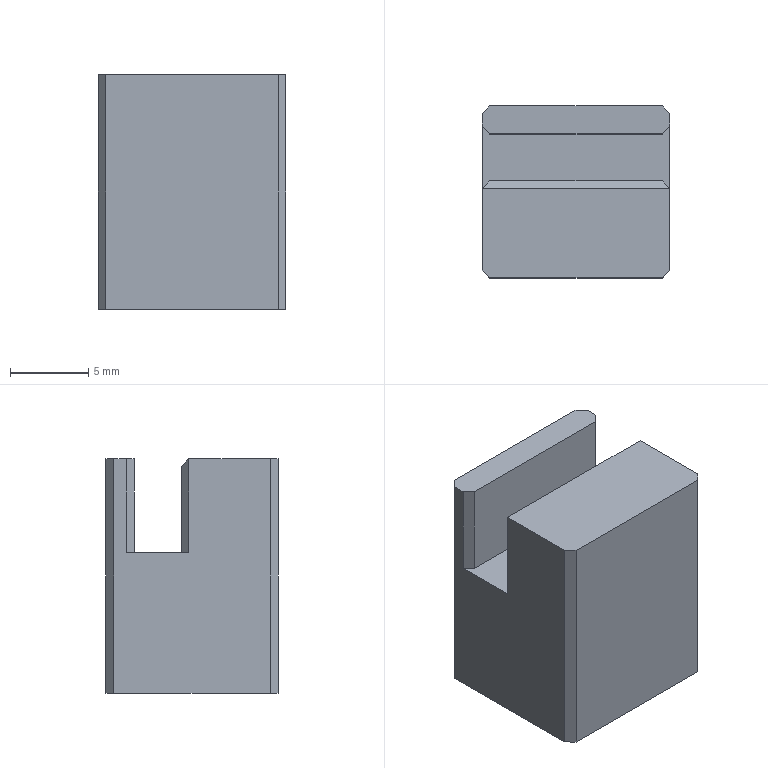Part | SolidWorks | features ICE 5, Chamfer 2, Extrusion 1 | 1 solid | 22 faces | box 12 x 11 x 15 mm | volume 1507 mm3 | plane 20 | cylinder 2 | commonest cylinder face diameters 5 x2
STEP:
#1=CARTESIAN_POINT('',(2.5,0.,5.));
#2=VERTEX_POINT('',#1);
#3=CARTESIAN_POINT('',(-2.5,0.,5.));
#4=VERTEX_POINT('',#3);
#5=CARTESIAN_POINT('',(0.,0.,5.));
#6=DIRECTION('',(0.,0.,-1.));
#7=DIRECTION('',(-1.,0.,0.));
#8=AXIS2_PLACEMENT_3D('',#5,#6,#7);
#9=CIRCLE('',#8,2.5);
#10=EDGE_CURVE('',#2,#4,#9,.T.);
#11=ORIENTED_EDGE('',*,*,#10,.F.);
#12=CARTESIAN_POINT('',(2.5,0.,-7.5));
#13=VERTEX_POINT('',#12);
#14=CARTESIAN_POINT('',(2.5,0.,5.));
#15=DIRECTION('',(0.,0.,-1.));
#16=VECTOR('',#15,1000.);
#17=LINE('',#14,#16);
#18=EDGE_CURVE('',#2,#13,#17,.T.);
#19=ORIENTED_EDGE('',*,*,#18,.T.);
#20=CARTESIAN_POINT('',(-2.5,0.,-7.5));
#21=VERTEX_POINT('',#20);
#22=CARTESIAN_POINT('',(0.,0.,-7.5));
#23=DIRECTION('',(0.,0.,-1.));
#24=DIRECTION('',(-1.,0.,0.));
#25=AXIS2_PLACEMENT_3D('',#22,#23,#24);
#26=CIRCLE('',#25,2.5);
#27=EDGE_CURVE('',#13,#21,#26,.T.);
#28=ORIENTED_EDGE('',*,*,#27,.T.);
#29=CARTESIAN_POINT('',(-2.5,0.,5.));
#30=DIRECTION('',(0.,0.,-1.));
#31=VECTOR('',#30,1000.);
#32=LINE('',#29,#31);
#33=EDGE_CURVE('',#4,#21,#32,.T.);
#34=ORIENTED_EDGE('',*,*,#33,.F.);
#35=EDGE_LOOP('',(#11,#19,#28,#34));
#36=FACE_OUTER_BOUND('',#35,.T.);
#37=CARTESIAN_POINT('',(0.,0.,5.));
#38=DIRECTION('',(0.,0.,-1.));
#39=DIRECTION('',(-1.,0.,0.));
#40=AXIS2_PLACEMENT_3D('',#37,#38,#39);
#41=CYLINDRICAL_SURFACE('',#40,2.5);
#42=ADVANCED_FACE('',(#36),#41,.F.);
#43=CARTESIAN_POINT('',(5.5,6.2,7.5));
#44=VERTEX_POINT('',#43);
#45=CARTESIAN_POINT('',(-5.5,6.2,7.5));
#46=VERTEX_POINT('',#45);
#47=CARTESIAN_POINT('',(-8.294,6.2,7.5));
#48=DIRECTION('',(-1.,0.,0.));
#49=VECTOR('',#48,1000.);
#50=LINE('',#47,#49);
#51=EDGE_CURVE('',#44,#46,#50,.T.);
#52=ORIENTED_EDGE('',*,*,#51,.F.);
#53=CARTESIAN_POINT('',(6.,6.7,7.5));
#54=VERTEX_POINT('',#53);
#55=CARTESIAN_POINT('',(-0.35,0.35,7.5));
#56=DIRECTION('',(0.7071,0.7071,0.));
#57=VECTOR('',#56,1000.);
#58=LINE('',#55,#57);
#59=EDGE_CURVE('',#44,#54,#58,.T.);
#60=ORIENTED_EDGE('',*,*,#59,.T.);
#61=CARTESIAN_POINT('',(6.,7.5,7.5));
#62=VERTEX_POINT('',#61);
#63=CARTESIAN_POINT('',(6.,-10.046,7.5));
#64=DIRECTION('',(0.,1.,0.));
#65=VECTOR('',#64,1000.);
#66=LINE('',#63,#65);
#67=EDGE_CURVE('',#54,#62,#66,.T.);
#68=ORIENTED_EDGE('',*,*,#67,.T.);
#69=CARTESIAN_POINT('',(5.5,8.,7.5));
#70=VERTEX_POINT('',#69);
#71=CARTESIAN_POINT('',(6.75,6.75,7.5));
#72=DIRECTION('',(-0.7071,0.7071,0.));
#73=VECTOR('',#72,1000.);
#74=LINE('',#71,#73);
#75=EDGE_CURVE('',#62,#70,#74,.T.);
#76=ORIENTED_EDGE('',*,*,#75,.T.);
#77=CARTESIAN_POINT('',(-5.5,8.,7.5));
#78=VERTEX_POINT('',#77);
#79=CARTESIAN_POINT('',(6.,8.,7.5));
#80=DIRECTION('',(1.,0.,0.));
#81=VECTOR('',#80,1000.);
#82=LINE('',#79,#81);
#83=EDGE_CURVE('',#78,#70,#82,.T.);
#84=ORIENTED_EDGE('',*,*,#83,.F.);
#85=CARTESIAN_POINT('',(-6.,7.5,7.5));
#86=VERTEX_POINT('',#85);
#87=CARTESIAN_POINT('',(-6.75,6.75,7.5));
#88=DIRECTION('',(-0.7071,-0.7071,0.));
#89=VECTOR('',#88,1000.);
#90=LINE('',#87,#89);
#91=EDGE_CURVE('',#78,#86,#90,.T.);
#92=ORIENTED_EDGE('',*,*,#91,.T.);
#93=CARTESIAN_POINT('',(-6.,6.7,7.5));
#94=VERTEX_POINT('',#93);
#95=CARTESIAN_POINT('',(-6.,-10.046,7.5));
#96=DIRECTION('',(0.,-1.,0.));
#97=VECTOR('',#96,1000.);
#98=LINE('',#95,#97);
#99=EDGE_CURVE('',#86,#94,#98,.T.);
#100=ORIENTED_EDGE('',*,*,#99,.T.);
#101=CARTESIAN_POINT('',(0.35,0.35,7.5));
#102=DIRECTION('',(0.7071,-0.7071,0.));
#103=VECTOR('',#102,1000.);
#104=LINE('',#101,#103);
#105=EDGE_CURVE('',#94,#46,#104,.T.);
#106=ORIENTED_EDGE('',*,*,#105,.T.);
#107=EDGE_LOOP('',(#52,#60,#68,#76,#84,#92,#100,#106));
#108=FACE_OUTER_BOUND('',#107,.T.);
#109=CARTESIAN_POINT('',(0.,0.,7.5));
#110=DIRECTION('',(0.,0.,1.));
#111=DIRECTION('',(1.,0.,0.));
#112=AXIS2_PLACEMENT_3D('',#109,#110,#111);
#113=PLANE('',#112);
#114=ADVANCED_FACE('',(#108),#113,.T.);
#115=CARTESIAN_POINT('',(6.,-2.5,7.5));
#116=VERTEX_POINT('',#115);
#117=CARTESIAN_POINT('',(6.,2.7,7.5));
#118=VERTEX_POINT('',#117);
#119=CARTESIAN_POINT('',(6.,-10.046,7.5));
#120=DIRECTION('',(0.,1.,0.));
#121=VECTOR('',#120,1000.);
#122=LINE('',#119,#121);
#123=EDGE_CURVE('',#116,#118,#122,.T.);
#124=ORIENTED_EDGE('',*,*,#123,.T.);
#125=CARTESIAN_POINT('',(-6.,2.7,7.5));
#126=VERTEX_POINT('',#125);
#127=CARTESIAN_POINT('',(-6.,2.7,7.5));
#128=DIRECTION('',(-1.,0.,0.));
#129=VECTOR('',#128,1000.);
#130=LINE('',#127,#129);
#131=EDGE_CURVE('',#118,#126,#130,.T.);
#132=ORIENTED_EDGE('',*,*,#131,.T.);
#133=CARTESIAN_POINT('',(-6.,-2.5,7.5));
#134=VERTEX_POINT('',#133);
#135=CARTESIAN_POINT('',(-6.,-10.046,7.5));
#136=DIRECTION('',(0.,-1.,0.));
#137=VECTOR('',#136,1000.);
#138=LINE('',#135,#137);
#139=EDGE_CURVE('',#126,#134,#138,.T.);
#140=ORIENTED_EDGE('',*,*,#139,.T.);
#141=CARTESIAN_POINT('',(-5.5,-3.,7.5));
#142=VERTEX_POINT('',#141);
#143=CARTESIAN_POINT('',(-4.25,-4.25,7.5));
#144=DIRECTION('',(0.7071,-0.7071,0.));
#145=VECTOR('',#144,1000.);
#146=LINE('',#143,#145);
#147=EDGE_CURVE('',#134,#142,#146,.T.);
#148=ORIENTED_EDGE('',*,*,#147,.T.);
#149=CARTESIAN_POINT('',(5.5,-3.,7.5));
#150=VERTEX_POINT('',#149);
#151=CARTESIAN_POINT('',(-7.853,-3.,7.5));
#152=DIRECTION('',(-1.,0.,0.));
#153=VECTOR('',#152,1000.);
#154=LINE('',#151,#153);
#155=EDGE_CURVE('',#150,#142,#154,.T.);
#156=ORIENTED_EDGE('',*,*,#155,.F.);
#157=CARTESIAN_POINT('',(4.25,-4.25,7.5));
#158=DIRECTION('',(0.7071,0.7071,0.));
#159=VECTOR('',#158,1000.);
#160=LINE('',#157,#159);
#161=EDGE_CURVE('',#150,#116,#160,.T.);
#162=ORIENTED_EDGE('',*,*,#161,.T.);
#163=EDGE_LOOP('',(#124,#132,#140,#148,#156,#162));
#164=FACE_OUTER_BOUND('',#163,.T.);
#165=CARTESIAN_POINT('',(0.,0.,7.5));
#166=DIRECTION('',(0.,0.,1.));
#167=DIRECTION('',(1.,0.,0.));
#168=AXIS2_PLACEMENT_3D('',#165,#166,#167);
#169=PLANE('',#168);
#170=ADVANCED_FACE('',(#164),#169,.T.);
#171=CARTESIAN_POINT('',(0.,0.,-7.5));
#172=DIRECTION('',(0.,0.,-1.));
#173=DIRECTION('',(-1.,0.,0.));
#174=AXIS2_PLACEMENT_3D('',#171,#172,#173);
#175=CIRCLE('',#174,2.5);
#176=EDGE_CURVE('',#21,#13,#175,.T.);
#177=ORIENTED_EDGE('',*,*,#176,.F.);
#178=ORIENTED_EDGE('',*,*,#27,.F.);
#179=EDGE_LOOP('',(#177,#178));
#180=FACE_BOUND('',#179,.T.);
#181=CARTESIAN_POINT('',(6.,-2.5,-7.5));
#182=VERTEX_POINT('',#181);
#183=CARTESIAN_POINT('',(6.,7.5,-7.5));
#184=VERTEX_POINT('',#183);
#185=CARTESIAN_POINT('',(6.,0.,-7.5));
#186=DIRECTION('',(0.,1.,0.));
#187=VECTOR('',#186,1000.);
#188=LINE('',#185,#187);
#189=EDGE_CURVE('',#182,#184,#188,.T.);
#190=ORIENTED_EDGE('',*,*,#189,.F.);
#191=CARTESIAN_POINT('',(5.5,-3.,-7.5));
#192=VERTEX_POINT('',#191);
#193=CARTESIAN_POINT('',(5.5,-3.,-7.5));
#194=DIRECTION('',(-0.7071,-0.7071,0.));
#195=VECTOR('',#194,1000.);
#196=LINE('',#193,#195);
#197=EDGE_CURVE('',#182,#192,#196,.T.);
#198=ORIENTED_EDGE('',*,*,#197,.T.);
#199=CARTESIAN_POINT('',(-5.5,-3.,-7.5));
#200=VERTEX_POINT('',#199);
#201=CARTESIAN_POINT('',(-7.853,-3.,-7.5));
#202=DIRECTION('',(-1.,0.,0.));
#203=VECTOR('',#202,1000.);
#204=LINE('',#201,#203);
#205=EDGE_CURVE('',#192,#200,#204,.T.);
#206=ORIENTED_EDGE('',*,*,#205,.T.);
#207=CARTESIAN_POINT('',(-6.,-2.5,-7.5));
#208=VERTEX_POINT('',#207);
#209=CARTESIAN_POINT('',(-5.5,-3.,-7.5));
#210=DIRECTION('',(-0.7071,0.7071,0.));
#211=VECTOR('',#210,1000.);
#212=LINE('',#209,#211);
#213=EDGE_CURVE('',#200,#208,#212,.T.);
#214=ORIENTED_EDGE('',*,*,#213,.T.);
#215=CARTESIAN_POINT('',(-6.,7.5,-7.5));
#216=VERTEX_POINT('',#215);
#217=CARTESIAN_POINT('',(-6.,0.,-7.5));
#218=DIRECTION('',(0.,-1.,0.));
#219=VECTOR('',#218,1000.);
#220=LINE('',#217,#219);
#221=EDGE_CURVE('',#216,#208,#220,.T.);
#222=ORIENTED_EDGE('',*,*,#221,.F.);
#223=CARTESIAN_POINT('',(-5.5,8.,-7.5));
#224=VERTEX_POINT('',#223);
#225=CARTESIAN_POINT('',(-6.,7.5,-7.5));
#226=DIRECTION('',(0.7071,0.7071,0.));
#227=VECTOR('',#226,1000.);
#228=LINE('',#225,#227);
#229=EDGE_CURVE('',#216,#224,#228,.T.);
#230=ORIENTED_EDGE('',*,*,#229,.T.);
#231=CARTESIAN_POINT('',(5.5,8.,-7.5));
#232=VERTEX_POINT('',#231);
#233=CARTESIAN_POINT('',(6.,8.,-7.5));
#234=DIRECTION('',(1.,0.,0.));
#235=VECTOR('',#234,1000.);
#236=LINE('',#233,#235);
#237=EDGE_CURVE('',#224,#232,#236,.T.);
#238=ORIENTED_EDGE('',*,*,#237,.T.);
#239=CARTESIAN_POINT('',(5.5,8.,-7.5));
#240=DIRECTION('',(0.7071,-0.7071,0.));
#241=VECTOR('',#240,1000.);
#242=LINE('',#239,#241);
#243=EDGE_CURVE('',#232,#184,#242,.T.);
#244=ORIENTED_EDGE('',*,*,#243,.T.);
#245=EDGE_LOOP('',(#190,#198,#206,#214,#222,#230,#238,#244));
#246=FACE_OUTER_BOUND('',#245,.T.);
#247=CARTESIAN_POINT('',(0.,0.,-7.5));
#248=DIRECTION('',(0.,0.,1.));
#249=DIRECTION('',(1.,0.,0.));
#250=AXIS2_PLACEMENT_3D('',#247,#248,#249);
#251=PLANE('',#250);
#252=ADVANCED_FACE('',(#180,#246),#251,.F.);
#253=ORIENTED_EDGE('',*,*,#18,.F.);
#254=CARTESIAN_POINT('',(0.,0.,5.));
#255=DIRECTION('',(0.,0.,-1.));
#256=DIRECTION('',(-1.,0.,0.));
#257=AXIS2_PLACEMENT_3D('',#254,#255,#256);
#258=CIRCLE('',#257,2.5);
#259=EDGE_CURVE('',#4,#2,#258,.T.);
#260=ORIENTED_EDGE('',*,*,#259,.F.);
#261=ORIENTED_EDGE('',*,*,#33,.T.);
#262=ORIENTED_EDGE('',*,*,#176,.T.);
#263=EDGE_LOOP('',(#253,#260,#261,#262));
#264=FACE_OUTER_BOUND('',#263,.T.);
#265=CARTESIAN_POINT('',(0.,0.,5.));
#266=DIRECTION('',(0.,0.,-1.));
#267=DIRECTION('',(-1.,0.,0.));
#268=AXIS2_PLACEMENT_3D('',#265,#266,#267);
#269=CYLINDRICAL_SURFACE('',#268,2.5);
#270=ADVANCED_FACE('',(#264),#269,.F.);
#271=ORIENTED_EDGE('',*,*,#259,.T.);
#272=ORIENTED_EDGE('',*,*,#10,.T.);
#273=EDGE_LOOP('',(#271,#272));
#274=FACE_OUTER_BOUND('',#273,.T.);
#275=CARTESIAN_POINT('',(0.,0.,5.));
#276=DIRECTION('',(0.,0.,-1.));
#277=DIRECTION('',(-1.,0.,0.));
#278=AXIS2_PLACEMENT_3D('',#275,#276,#277);
#279=PLANE('',#278);
#280=ADVANCED_FACE('',(#274),#279,.T.);
#281=CARTESIAN_POINT('',(-6.,2.7,1.5));
#282=VERTEX_POINT('',#281);
#283=CARTESIAN_POINT('',(-6.,6.7,1.5));
#284=VERTEX_POINT('',#283);
#285=CARTESIAN_POINT('',(-6.,-10.046,1.5));
#286=DIRECTION('',(0.,1.,0.));
#287=VECTOR('',#286,1000.);
#288=LINE('',#285,#287);
#289=EDGE_CURVE('',#282,#284,#288,.T.);
#290=ORIENTED_EDGE('',*,*,#289,.T.);
#291=CARTESIAN_POINT('',(-6.,6.7,7.5));
#292=DIRECTION('',(0.,0.,1.));
#293=VECTOR('',#292,1000.);
#294=LINE('',#291,#293);
#295=EDGE_CURVE('',#284,#94,#294,.T.);
#296=ORIENTED_EDGE('',*,*,#295,.T.);
#297=ORIENTED_EDGE('',*,*,#99,.F.);
#298=CARTESIAN_POINT('',(-6.,7.5,-7.5));
#299=DIRECTION('',(0.,0.,-1.));
#300=VECTOR('',#299,1000.);
#301=LINE('',#298,#300);
#302=EDGE_CURVE('',#86,#216,#301,.T.);
#303=ORIENTED_EDGE('',*,*,#302,.T.);
#304=ORIENTED_EDGE('',*,*,#221,.T.);
#305=CARTESIAN_POINT('',(-6.,-2.5,7.5));
#306=DIRECTION('',(0.,0.,1.));
#307=VECTOR('',#306,1000.);
#308=LINE('',#305,#307);
#309=EDGE_CURVE('',#208,#134,#308,.T.);
#310=ORIENTED_EDGE('',*,*,#309,.T.);
#311=ORIENTED_EDGE('',*,*,#139,.F.);
#312=CARTESIAN_POINT('',(-6.,2.7,1.5));
#313=DIRECTION('',(0.,0.,-1.));
#314=VECTOR('',#313,1000.);
#315=LINE('',#312,#314);
#316=EDGE_CURVE('',#126,#282,#315,.T.);
#317=ORIENTED_EDGE('',*,*,#316,.T.);
#318=EDGE_LOOP('',(#290,#296,#297,#303,#304,#310,#311,#317));
#319=FACE_OUTER_BOUND('',#318,.T.);
#320=CARTESIAN_POINT('',(-6.,-10.046,-7.5));
#321=DIRECTION('',(-1.,0.,0.));
#322=DIRECTION('',(0.,0.,1.));
#323=AXIS2_PLACEMENT_3D('',#320,#321,#322);
#324=PLANE('',#323);
#325=ADVANCED_FACE('',(#319),#324,.T.);
#326=ORIENTED_EDGE('',*,*,#67,.F.);
#327=CARTESIAN_POINT('',(6.,6.7,1.5));
#328=VERTEX_POINT('',#327);
#329=CARTESIAN_POINT('',(6.,6.7,1.5));
#330=DIRECTION('',(0.,0.,-1.));
#331=VECTOR('',#330,1000.);
#332=LINE('',#329,#331);
#333=EDGE_CURVE('',#54,#328,#332,.T.);
#334=ORIENTED_EDGE('',*,*,#333,.T.);
#335=CARTESIAN_POINT('',(6.,2.7,1.5));
#336=VERTEX_POINT('',#335);
#337=CARTESIAN_POINT('',(6.,-10.046,1.5));
#338=DIRECTION('',(0.,-1.,0.));
#339=VECTOR('',#338,1000.);
#340=LINE('',#337,#339);
#341=EDGE_CURVE('',#328,#336,#340,.T.);
#342=ORIENTED_EDGE('',*,*,#341,.T.);
#343=CARTESIAN_POINT('',(6.,2.7,7.5));
#344=DIRECTION('',(0.,0.,1.));
#345=VECTOR('',#344,1000.);
#346=LINE('',#343,#345);
#347=EDGE_CURVE('',#336,#118,#346,.T.);
#348=ORIENTED_EDGE('',*,*,#347,.T.);
#349=ORIENTED_EDGE('',*,*,#123,.F.);
#350=CARTESIAN_POINT('',(6.,-2.5,-7.5));
#351=DIRECTION('',(0.,0.,-1.));
#352=VECTOR('',#351,1000.);
#353=LINE('',#350,#352);
#354=EDGE_CURVE('',#116,#182,#353,.T.);
#355=ORIENTED_EDGE('',*,*,#354,.T.);
#356=ORIENTED_EDGE('',*,*,#189,.T.);
#357=CARTESIAN_POINT('',(6.,7.5,-7.5));
#358=DIRECTION('',(0.,0.,1.));
#359=VECTOR('',#358,1000.);
#360=LINE('',#357,#359);
#361=EDGE_CURVE('',#184,#62,#360,.T.);
#362=ORIENTED_EDGE('',*,*,#361,.T.);
#363=EDGE_LOOP('',(#326,#334,#342,#348,#349,#355,#356,#362));
#364=FACE_OUTER_BOUND('',#363,.T.);
#365=CARTESIAN_POINT('',(6.,-10.046,-7.5));
#366=DIRECTION('',(1.,0.,0.));
#367=DIRECTION('',(0.,0.,-1.));
#368=AXIS2_PLACEMENT_3D('',#365,#366,#367);
#369=PLANE('',#368);
#370=ADVANCED_FACE('',(#364),#369,.T.);
#371=ORIENTED_EDGE('',*,*,#205,.F.);
#372=CARTESIAN_POINT('',(5.5,-3.,7.5));
#373=DIRECTION('',(0.,0.,1.));
#374=VECTOR('',#373,1000.);
#375=LINE('',#372,#374);
#376=EDGE_CURVE('',#192,#150,#375,.T.);
#377=ORIENTED_EDGE('',*,*,#376,.T.);
#378=ORIENTED_EDGE('',*,*,#155,.T.);
#379=CARTESIAN_POINT('',(-5.5,-3.,-7.5));
#380=DIRECTION('',(0.,0.,-1.));
#381=VECTOR('',#380,1000.);
#382=LINE('',#379,#381);
#383=EDGE_CURVE('',#142,#200,#382,.T.);
#384=ORIENTED_EDGE('',*,*,#383,.T.);
#385=EDGE_LOOP('',(#371,#377,#378,#384));
#386=FACE_OUTER_BOUND('',#385,.T.);
#387=CARTESIAN_POINT('',(-7.853,-3.,-7.5));
#388=DIRECTION('',(0.,1.,0.));
#389=DIRECTION('',(0.,0.,1.));
#390=AXIS2_PLACEMENT_3D('',#387,#388,#389);
#391=PLANE('',#390);
#392=ADVANCED_FACE('',(#386),#391,.F.);
#393=ORIENTED_EDGE('',*,*,#237,.F.);
#394=CARTESIAN_POINT('',(-5.5,8.,19.802));
#395=DIRECTION('',(0.,0.,1.));
#396=VECTOR('',#395,1000.);
#397=LINE('',#394,#396);
#398=EDGE_CURVE('',#224,#78,#397,.T.);
#399=ORIENTED_EDGE('',*,*,#398,.T.);
#400=ORIENTED_EDGE('',*,*,#83,.T.);
#401=CARTESIAN_POINT('',(5.5,8.,19.802));
#402=DIRECTION('',(0.,0.,-1.));
#403=VECTOR('',#402,1000.);
#404=LINE('',#401,#403);
#405=EDGE_CURVE('',#70,#232,#404,.T.);
#406=ORIENTED_EDGE('',*,*,#405,.T.);
#407=EDGE_LOOP('',(#393,#399,#400,#406));
#408=FACE_OUTER_BOUND('',#407,.T.);
#409=CARTESIAN_POINT('',(6.,8.,19.802));
#410=DIRECTION('',(0.,1.,0.));
#411=DIRECTION('',(0.,0.,1.));
#412=AXIS2_PLACEMENT_3D('',#409,#410,#411);
#413=PLANE('',#412);
#414=ADVANCED_FACE('',(#408),#413,.T.);
#415=ORIENTED_EDGE('',*,*,#197,.F.);
#416=ORIENTED_EDGE('',*,*,#354,.F.);
#417=ORIENTED_EDGE('',*,*,#161,.F.);
#418=ORIENTED_EDGE('',*,*,#376,.F.);
#419=EDGE_LOOP('',(#415,#416,#417,#418));
#420=FACE_OUTER_BOUND('',#419,.T.);
#421=CARTESIAN_POINT('',(5.5,-3.,-7.5));
#422=DIRECTION('',(0.7071,-0.7071,0.));
#423=DIRECTION('',(0.,0.,-1.));
#424=AXIS2_PLACEMENT_3D('',#421,#422,#423);
#425=PLANE('',#424);
#426=ADVANCED_FACE('',(#420),#425,.T.);
#427=ORIENTED_EDGE('',*,*,#147,.F.);
#428=ORIENTED_EDGE('',*,*,#309,.F.);
#429=ORIENTED_EDGE('',*,*,#213,.F.);
#430=ORIENTED_EDGE('',*,*,#383,.F.);
#431=EDGE_LOOP('',(#427,#428,#429,#430));
#432=FACE_OUTER_BOUND('',#431,.T.);
#433=CARTESIAN_POINT('',(-5.5,-3.,-7.5));
#434=DIRECTION('',(-0.7071,-0.7071,0.));
#435=DIRECTION('',(0.,0.,1.));
#436=AXIS2_PLACEMENT_3D('',#433,#434,#435);
#437=PLANE('',#436);
#438=ADVANCED_FACE('',(#432),#437,.T.);
#439=ORIENTED_EDGE('',*,*,#91,.F.);
#440=ORIENTED_EDGE('',*,*,#398,.F.);
#441=ORIENTED_EDGE('',*,*,#229,.F.);
#442=ORIENTED_EDGE('',*,*,#302,.F.);
#443=EDGE_LOOP('',(#439,#440,#441,#442));
#444=FACE_OUTER_BOUND('',#443,.T.);
#445=CARTESIAN_POINT('',(-6.,7.5,-7.5));
#446=DIRECTION('',(0.7071,-0.7071,0.));
#447=DIRECTION('',(0.,0.,-1.));
#448=AXIS2_PLACEMENT_3D('',#445,#446,#447);
#449=PLANE('',#448);
#450=ADVANCED_FACE('',(#444),#449,.F.);
#451=ORIENTED_EDGE('',*,*,#75,.F.);
#452=ORIENTED_EDGE('',*,*,#361,.F.);
#453=ORIENTED_EDGE('',*,*,#243,.F.);
#454=ORIENTED_EDGE('',*,*,#405,.F.);
#455=EDGE_LOOP('',(#451,#452,#453,#454));
#456=FACE_OUTER_BOUND('',#455,.T.);
#457=CARTESIAN_POINT('',(5.5,8.,19.802));
#458=DIRECTION('',(-0.7071,-0.7071,0.));
#459=DIRECTION('',(0.,0.,-1.));
#460=AXIS2_PLACEMENT_3D('',#457,#458,#459);
#461=PLANE('',#460);
#462=ADVANCED_FACE('',(#456),#461,.F.);
#463=CARTESIAN_POINT('',(5.5,6.2,1.5));
#464=VERTEX_POINT('',#463);
#465=CARTESIAN_POINT('',(-5.5,6.2,1.5));
#466=VERTEX_POINT('',#465);
#467=CARTESIAN_POINT('',(-8.294,6.2,1.5));
#468=DIRECTION('',(-1.,0.,0.));
#469=VECTOR('',#468,1000.);
#470=LINE('',#467,#469);
#471=EDGE_CURVE('',#464,#466,#470,.T.);
#472=ORIENTED_EDGE('',*,*,#471,.F.);
#473=CARTESIAN_POINT('',(5.5,6.2,7.5));
#474=DIRECTION('',(0.,0.,1.));
#475=VECTOR('',#474,1000.);
#476=LINE('',#473,#475);
#477=EDGE_CURVE('',#464,#44,#476,.T.);
#478=ORIENTED_EDGE('',*,*,#477,.T.);
#479=ORIENTED_EDGE('',*,*,#51,.T.);
#480=CARTESIAN_POINT('',(-5.5,6.2,1.5));
#481=DIRECTION('',(0.,0.,-1.));
#482=VECTOR('',#481,1000.);
#483=LINE('',#480,#482);
#484=EDGE_CURVE('',#46,#466,#483,.T.);
#485=ORIENTED_EDGE('',*,*,#484,.T.);
#486=EDGE_LOOP('',(#472,#478,#479,#485));
#487=FACE_OUTER_BOUND('',#486,.T.);
#488=CARTESIAN_POINT('',(-8.294,6.2,1.5));
#489=DIRECTION('',(0.,1.,0.));
#490=DIRECTION('',(0.,0.,1.));
#491=AXIS2_PLACEMENT_3D('',#488,#489,#490);
#492=PLANE('',#491);
#493=ADVANCED_FACE('',(#487),#492,.F.);
#494=CARTESIAN_POINT('',(-5.5,3.2,7.));
#495=VERTEX_POINT('',#494);
#496=CARTESIAN_POINT('',(5.5,3.2,7.));
#497=VERTEX_POINT('',#496);
#498=CARTESIAN_POINT('',(6.,3.2,7.));
#499=DIRECTION('',(1.,0.,0.));
#500=VECTOR('',#499,1000.);
#501=LINE('',#498,#500);
#502=EDGE_CURVE('',#495,#497,#501,.T.);
#503=ORIENTED_EDGE('',*,*,#502,.T.);
#504=CARTESIAN_POINT('',(5.5,3.2,1.5));
#505=VERTEX_POINT('',#504);
#506=CARTESIAN_POINT('',(5.5,3.2,1.5));
#507=DIRECTION('',(0.,0.,-1.));
#508=VECTOR('',#507,1000.);
#509=LINE('',#506,#508);
#510=EDGE_CURVE('',#497,#505,#509,.T.);
#511=ORIENTED_EDGE('',*,*,#510,.T.);
#512=CARTESIAN_POINT('',(-5.5,3.2,1.5));
#513=VERTEX_POINT('',#512);
#514=CARTESIAN_POINT('',(-8.294,3.2,1.5));
#515=DIRECTION('',(1.,0.,0.));
#516=VECTOR('',#515,1000.);
#517=LINE('',#514,#516);
#518=EDGE_CURVE('',#513,#505,#517,.T.);
#519=ORIENTED_EDGE('',*,*,#518,.F.);
#520=CARTESIAN_POINT('',(-5.5,3.2,7.5));
#521=DIRECTION('',(0.,0.,1.));
#522=VECTOR('',#521,1000.);
#523=LINE('',#520,#522);
#524=EDGE_CURVE('',#513,#495,#523,.T.);
#525=ORIENTED_EDGE('',*,*,#524,.T.);
#526=EDGE_LOOP('',(#503,#511,#519,#525));
#527=FACE_OUTER_BOUND('',#526,.T.);
#528=CARTESIAN_POINT('',(-8.294,3.2,1.5));
#529=DIRECTION('',(0.,-1.,0.));
#530=DIRECTION('',(0.,0.,-1.));
#531=AXIS2_PLACEMENT_3D('',#528,#529,#530);
#532=PLANE('',#531);
#533=ADVANCED_FACE('',(#527),#532,.F.);
#534=ORIENTED_EDGE('',*,*,#289,.F.);
#535=CARTESIAN_POINT('',(-5.5,3.2,1.5));
#536=DIRECTION('',(0.7071,0.7071,0.));
#537=VECTOR('',#536,1000.);
#538=LINE('',#535,#537);
#539=EDGE_CURVE('',#282,#513,#538,.T.);
#540=ORIENTED_EDGE('',*,*,#539,.T.);
#541=ORIENTED_EDGE('',*,*,#518,.T.);
#542=CARTESIAN_POINT('',(5.5,3.2,1.5));
#543=DIRECTION('',(0.7071,-0.7071,0.));
#544=VECTOR('',#543,1000.);
#545=LINE('',#542,#544);
#546=EDGE_CURVE('',#505,#336,#545,.T.);
#547=ORIENTED_EDGE('',*,*,#546,.T.);
#548=ORIENTED_EDGE('',*,*,#341,.F.);
#549=CARTESIAN_POINT('',(5.5,6.2,1.5));
#550=DIRECTION('',(-0.7071,-0.7071,0.));
#551=VECTOR('',#550,1000.);
#552=LINE('',#549,#551);
#553=EDGE_CURVE('',#328,#464,#552,.T.);
#554=ORIENTED_EDGE('',*,*,#553,.T.);
#555=ORIENTED_EDGE('',*,*,#471,.T.);
#556=CARTESIAN_POINT('',(-5.5,6.2,1.5));
#557=DIRECTION('',(-0.7071,0.7071,0.));
#558=VECTOR('',#557,1000.);
#559=LINE('',#556,#558);
#560=EDGE_CURVE('',#466,#284,#559,.T.);
#561=ORIENTED_EDGE('',*,*,#560,.T.);
#562=EDGE_LOOP('',(#534,#540,#541,#547,#548,#554,#555,#561));
#563=FACE_OUTER_BOUND('',#562,.T.);
#564=CARTESIAN_POINT('',(0.,0.,1.5));
#565=DIRECTION('',(0.,0.,1.));
#566=DIRECTION('',(1.,0.,0.));
#567=AXIS2_PLACEMENT_3D('',#564,#565,#566);
#568=PLANE('',#567);
#569=ADVANCED_FACE('',(#563),#568,.T.);
#570=ORIENTED_EDGE('',*,*,#553,.F.);
#571=ORIENTED_EDGE('',*,*,#333,.F.);
#572=ORIENTED_EDGE('',*,*,#59,.F.);
#573=ORIENTED_EDGE('',*,*,#477,.F.);
#574=EDGE_LOOP('',(#570,#571,#572,#573));
#575=FACE_OUTER_BOUND('',#574,.T.);
#576=CARTESIAN_POINT('',(5.5,6.2,1.5));
#577=DIRECTION('',(0.7071,-0.7071,0.));
#578=DIRECTION('',(0.,0.,-1.));
#579=AXIS2_PLACEMENT_3D('',#576,#577,#578);
#580=PLANE('',#579);
#581=ADVANCED_FACE('',(#575),#580,.T.);
#582=ORIENTED_EDGE('',*,*,#105,.F.);
#583=ORIENTED_EDGE('',*,*,#295,.F.);
#584=ORIENTED_EDGE('',*,*,#560,.F.);
#585=ORIENTED_EDGE('',*,*,#484,.F.);
#586=EDGE_LOOP('',(#582,#583,#584,#585));
#587=FACE_OUTER_BOUND('',#586,.T.);
#588=CARTESIAN_POINT('',(-5.5,6.2,1.5));
#589=DIRECTION('',(-0.7071,-0.7071,0.));
#590=DIRECTION('',(0.,0.,1.));
#591=AXIS2_PLACEMENT_3D('',#588,#589,#590);
#592=PLANE('',#591);
#593=ADVANCED_FACE('',(#587),#592,.T.);
#594=ORIENTED_EDGE('',*,*,#539,.F.);
#595=ORIENTED_EDGE('',*,*,#316,.F.);
#596=CARTESIAN_POINT('',(-3.667,5.033,5.167));
#597=DIRECTION('',(-0.5774,-0.5774,0.5774));
#598=VECTOR('',#597,1000.);
#599=LINE('',#596,#598);
#600=EDGE_CURVE('',#495,#126,#599,.T.);
#601=ORIENTED_EDGE('',*,*,#600,.F.);
#602=ORIENTED_EDGE('',*,*,#524,.F.);
#603=EDGE_LOOP('',(#594,#595,#601,#602));
#604=FACE_OUTER_BOUND('',#603,.T.);
#605=CARTESIAN_POINT('',(-5.5,3.2,1.5));
#606=DIRECTION('',(-0.7071,0.7071,0.));
#607=DIRECTION('',(0.,0.,-1.));
#608=AXIS2_PLACEMENT_3D('',#605,#606,#607);
#609=PLANE('',#608);
#610=ADVANCED_FACE('',(#604),#609,.T.);
#611=ORIENTED_EDGE('',*,*,#600,.T.);
#612=ORIENTED_EDGE('',*,*,#131,.F.);
#613=CARTESIAN_POINT('',(0.9021,7.798,2.402));
#614=DIRECTION('',(0.5774,-0.5774,0.5774));
#615=VECTOR('',#614,1000.);
#616=LINE('',#613,#615);
#617=EDGE_CURVE('',#497,#118,#616,.T.);
#618=ORIENTED_EDGE('',*,*,#617,.F.);
#619=ORIENTED_EDGE('',*,*,#502,.F.);
#620=EDGE_LOOP('',(#611,#612,#618,#619));
#621=FACE_OUTER_BOUND('',#620,.T.);
#622=CARTESIAN_POINT('',(-8.294,3.2,7.));
#623=DIRECTION('',(0.,0.7071,0.7071));
#624=DIRECTION('',(-1.,0.,0.));
#625=AXIS2_PLACEMENT_3D('',#622,#623,#624);
#626=PLANE('',#625);
#627=ADVANCED_FACE('',(#621),#626,.T.);
#628=ORIENTED_EDGE('',*,*,#617,.T.);
#629=ORIENTED_EDGE('',*,*,#347,.F.);
#630=ORIENTED_EDGE('',*,*,#546,.F.);
#631=ORIENTED_EDGE('',*,*,#510,.F.);
#632=EDGE_LOOP('',(#628,#629,#630,#631));
#633=FACE_OUTER_BOUND('',#632,.T.);
#634=CARTESIAN_POINT('',(5.5,3.2,1.5));
#635=DIRECTION('',(0.7071,0.7071,0.));
#636=DIRECTION('',(0.,0.,1.));
#637=AXIS2_PLACEMENT_3D('',#634,#635,#636);
#638=PLANE('',#637);
#639=ADVANCED_FACE('',(#633),#638,.T.);
#640=CLOSED_SHELL('',(#42,#114,#170,#252,#270,#280,#325,#370,#392,#414,#426,#438,#450,#462,#493,#533,#569,#581,#593,#610,#627,#639));
#641=MANIFOLD_SOLID_BREP('',#640);
#642=CARTESIAN_POINT('',(0.,0.,0.));
#643=DIRECTION('',(0.,0.,1.));
#644=DIRECTION('',(1.,0.,0.));
#645=AXIS2_PLACEMENT_3D('',#642,#643,#644);
#646=(LENGTH_UNIT()NAMED_UNIT(*)SI_UNIT(.MILLI.,.METRE.));
#647=UNCERTAINTY_MEASURE_WITH_UNIT(LENGTH_MEASURE(0.00001),#646,'','');
#648=(NAMED_UNIT(*)PLANE_ANGLE_UNIT()SI_UNIT($,.RADIAN.));
#649=(NAMED_UNIT(*)SI_UNIT($,.STERADIAN.)SOLID_ANGLE_UNIT());
#650=(GEOMETRIC_REPRESENTATION_CONTEXT(3)GLOBAL_UNCERTAINTY_ASSIGNED_CONTEXT((#647))GLOBAL_UNIT_ASSIGNED_CONTEXT((#646,#648,#649))REPRESENTATION_CONTEXT('',''));
#651=ADVANCED_BREP_SHAPE_REPRESENTATION('',(#641,#645),#650);